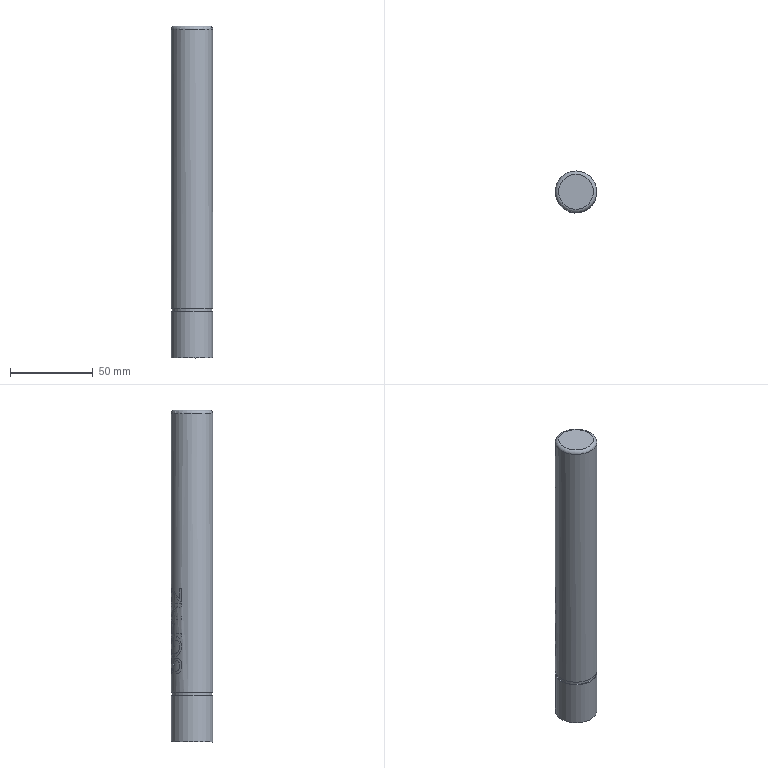Part | NX | features SGPN25-140_1 2 | 1 solid | 87 faces | box 25 x 25.002 x 200 mm | volume 96902 mm3 | plane 48 | cylinder 36 | cone 2 | torus 1 | commonest cylinder face diameters 24.8 x5 25 x3 3.389 x1 3.509 x1 4.336 x1 4.656 x1